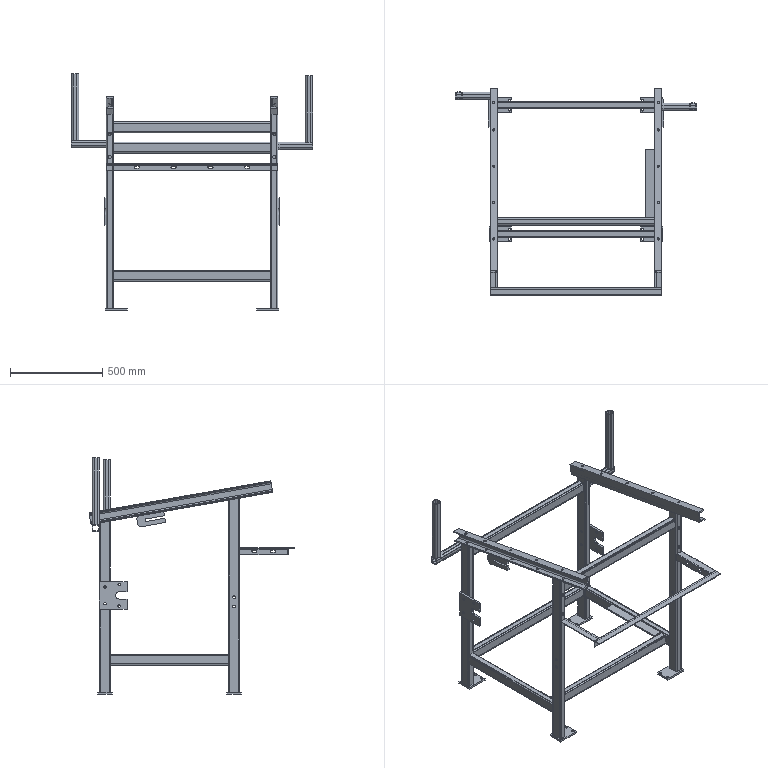Part | SolidWorks | features LayoutProfileFeature 1 | 27 solids | 531 faces | box 1308 x 1116 x 1280 mm | volume 8216576 mm3 | cylinder 272 | plane 259 | commonest cylinder face diameters 13 x108 15 x60 9 x40 16 x16 17 x16 24 x16